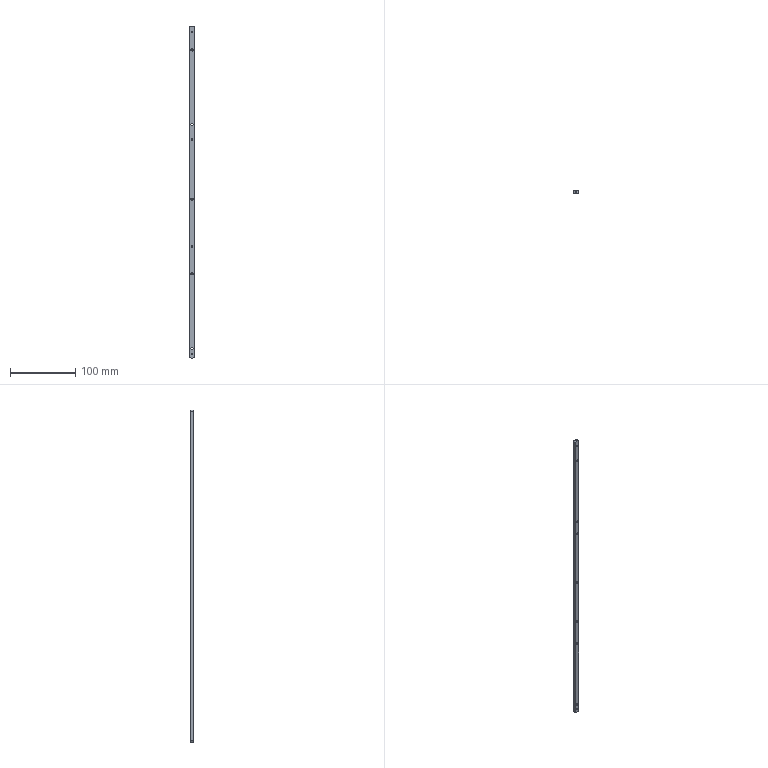Part | NX | 1 solid | 33 faces | box 7 x 5 x 507 mm | volume 17027 mm3 | cylinder 18 | plane 11 | cone 4 | commonest cylinder face diameters 3.4 x5 6 x5 2.5 x4 4 x4
STEP:
#1=CARTESIAN_POINT('',(0.,1.6,220.));
#2=VERTEX_POINT('',#1);
#3=CARTESIAN_POINT('',(0.,1.6,217.));
#4=DIRECTION('',(0.,1.,0.));
#5=DIRECTION('',(0.,0.,1.));
#6=AXIS2_PLACEMENT_3D('',#3,#4,#5);
#7=CIRCLE('',#6,3.);
#8=EDGE_CURVE('',#2,#2,#7,.T.);
#9=ORIENTED_EDGE('',*,*,#8,.T.);
#10=EDGE_LOOP('',(#9));
#11=FACE_BOUND('',#10,.T.);
#12=CARTESIAN_POINT('',(0.,1.6,218.7));
#13=VERTEX_POINT('',#12);
#14=CARTESIAN_POINT('',(0.,1.6,217.));
#15=DIRECTION('',(0.,1.,0.));
#16=DIRECTION('',(0.,0.,1.));
#17=AXIS2_PLACEMENT_3D('',#14,#15,#16);
#18=CIRCLE('',#17,1.7);
#19=EDGE_CURVE('',#13,#13,#18,.T.);
#20=ORIENTED_EDGE('',*,*,#19,.F.);
#21=EDGE_LOOP('',(#20));
#22=FACE_BOUND('',#21,.T.);
#23=CARTESIAN_POINT('',(1.7,1.6,217.));
#24=DIRECTION('',(0.,-1.,0.));
#25=DIRECTION('',(0.,0.,-1.));
#26=AXIS2_PLACEMENT_3D('',#23,#24,#25);
#27=PLANE('',#26);
#28=ADVANCED_FACE('',(#11,#22),#27,.F.);
#29=CARTESIAN_POINT('',(0.,1.6,100.));
#30=VERTEX_POINT('',#29);
#31=CARTESIAN_POINT('',(0.,1.6,103.));
#32=DIRECTION('',(0.,1.,0.));
#33=DIRECTION('',(0.,0.,-1.));
#34=AXIS2_PLACEMENT_3D('',#31,#32,#33);
#35=CIRCLE('',#34,3.);
#36=EDGE_CURVE('',#30,#30,#35,.T.);
#37=ORIENTED_EDGE('',*,*,#36,.T.);
#38=EDGE_LOOP('',(#37));
#39=FACE_BOUND('',#38,.T.);
#40=CARTESIAN_POINT('',(0.,1.6,101.3));
#41=VERTEX_POINT('',#40);
#42=CARTESIAN_POINT('',(0.,1.6,103.));
#43=DIRECTION('',(0.,1.,0.));
#44=DIRECTION('',(0.,0.,-1.));
#45=AXIS2_PLACEMENT_3D('',#42,#43,#44);
#46=CIRCLE('',#45,1.7);
#47=EDGE_CURVE('',#41,#41,#46,.T.);
#48=ORIENTED_EDGE('',*,*,#47,.F.);
#49=EDGE_LOOP('',(#48));
#50=FACE_BOUND('',#49,.T.);
#51=CARTESIAN_POINT('',(1.7,1.6,217.));
#52=DIRECTION('',(0.,-1.,0.));
#53=DIRECTION('',(0.,0.,-1.));
#54=AXIS2_PLACEMENT_3D('',#51,#52,#53);
#55=PLANE('',#54);
#56=ADVANCED_FACE('',(#39,#50),#55,.F.);
#57=CARTESIAN_POINT('',(0.,1.6,-14.));
#58=VERTEX_POINT('',#57);
#59=CARTESIAN_POINT('',(0.,1.6,-11.));
#60=DIRECTION('',(0.,1.,0.));
#61=DIRECTION('',(0.,0.,-1.));
#62=AXIS2_PLACEMENT_3D('',#59,#60,#61);
#63=CIRCLE('',#62,3.);
#64=EDGE_CURVE('',#58,#58,#63,.T.);
#65=ORIENTED_EDGE('',*,*,#64,.T.);
#66=EDGE_LOOP('',(#65));
#67=FACE_BOUND('',#66,.T.);
#68=CARTESIAN_POINT('',(0.,1.6,-12.7));
#69=VERTEX_POINT('',#68);
#70=CARTESIAN_POINT('',(0.,1.6,-11.));
#71=DIRECTION('',(0.,1.,0.));
#72=DIRECTION('',(0.,0.,-1.));
#73=AXIS2_PLACEMENT_3D('',#70,#71,#72);
#74=CIRCLE('',#73,1.7);
#75=EDGE_CURVE('',#69,#69,#74,.T.);
#76=ORIENTED_EDGE('',*,*,#75,.F.);
#77=EDGE_LOOP('',(#76));
#78=FACE_BOUND('',#77,.T.);
#79=CARTESIAN_POINT('',(1.7,1.6,217.));
#80=DIRECTION('',(0.,-1.,0.));
#81=DIRECTION('',(0.,0.,-1.));
#82=AXIS2_PLACEMENT_3D('',#79,#80,#81);
#83=PLANE('',#82);
#84=ADVANCED_FACE('',(#67,#78),#83,.F.);
#85=CARTESIAN_POINT('',(0.,1.6,-128.));
#86=VERTEX_POINT('',#85);
#87=CARTESIAN_POINT('',(0.,1.6,-125.));
#88=DIRECTION('',(0.,1.,0.));
#89=DIRECTION('',(0.,0.,-1.));
#90=AXIS2_PLACEMENT_3D('',#87,#88,#89);
#91=CIRCLE('',#90,3.);
#92=EDGE_CURVE('',#86,#86,#91,.T.);
#93=ORIENTED_EDGE('',*,*,#92,.T.);
#94=EDGE_LOOP('',(#93));
#95=FACE_BOUND('',#94,.T.);
#96=CARTESIAN_POINT('',(0.,1.6,-126.7));
#97=VERTEX_POINT('',#96);
#98=CARTESIAN_POINT('',(0.,1.6,-125.));
#99=DIRECTION('',(0.,1.,0.));
#100=DIRECTION('',(0.,0.,-1.));
#101=AXIS2_PLACEMENT_3D('',#98,#99,#100);
#102=CIRCLE('',#101,1.7);
#103=EDGE_CURVE('',#97,#97,#102,.T.);
#104=ORIENTED_EDGE('',*,*,#103,.F.);
#105=EDGE_LOOP('',(#104));
#106=FACE_BOUND('',#105,.T.);
#107=CARTESIAN_POINT('',(1.7,1.6,217.));
#108=DIRECTION('',(0.,-1.,0.));
#109=DIRECTION('',(0.,0.,-1.));
#110=AXIS2_PLACEMENT_3D('',#107,#108,#109);
#111=PLANE('',#110);
#112=ADVANCED_FACE('',(#95,#106),#111,.F.);
#113=CARTESIAN_POINT('',(0.,1.6,-242.));
#114=VERTEX_POINT('',#113);
#115=CARTESIAN_POINT('',(0.,1.6,-239.));
#116=DIRECTION('',(0.,1.,0.));
#117=DIRECTION('',(0.,0.,-1.));
#118=AXIS2_PLACEMENT_3D('',#115,#116,#117);
#119=CIRCLE('',#118,3.);
#120=EDGE_CURVE('',#114,#114,#119,.T.);
#121=ORIENTED_EDGE('',*,*,#120,.T.);
#122=EDGE_LOOP('',(#121));
#123=FACE_BOUND('',#122,.T.);
#124=CARTESIAN_POINT('',(0.,1.6,-240.7));
#125=VERTEX_POINT('',#124);
#126=CARTESIAN_POINT('',(0.,1.6,-239.));
#127=DIRECTION('',(0.,1.,0.));
#128=DIRECTION('',(0.,0.,-1.));
#129=AXIS2_PLACEMENT_3D('',#126,#127,#128);
#130=CIRCLE('',#129,1.7);
#131=EDGE_CURVE('',#125,#125,#130,.T.);
#132=ORIENTED_EDGE('',*,*,#131,.F.);
#133=EDGE_LOOP('',(#132));
#134=FACE_BOUND('',#133,.T.);
#135=CARTESIAN_POINT('',(1.7,1.6,217.));
#136=DIRECTION('',(0.,-1.,0.));
#137=DIRECTION('',(0.,0.,-1.));
#138=AXIS2_PLACEMENT_3D('',#135,#136,#137);
#139=PLANE('',#138);
#140=ADVANCED_FACE('',(#123,#134),#139,.F.);
#141=CARTESIAN_POINT('',(-3.5,5.,251.5));
#142=VERTEX_POINT('',#141);
#143=CARTESIAN_POINT('',(-1.5,5.,253.5));
#144=VERTEX_POINT('',#143);
#145=CARTESIAN_POINT('',(-1.5,5.,251.5));
#146=DIRECTION('',(0.,1.,0.));
#147=DIRECTION('',(0.,0.,1.));
#148=AXIS2_PLACEMENT_3D('',#145,#146,#147);
#149=CIRCLE('',#148,2.);
#150=EDGE_CURVE('',#142,#144,#149,.T.);
#151=ORIENTED_EDGE('',*,*,#150,.F.);
#152=CARTESIAN_POINT('',(-3.5,0.,251.5));
#153=VERTEX_POINT('',#152);
#154=CARTESIAN_POINT('',(-3.5,5.,251.5));
#155=DIRECTION('',(0.,1.,0.));
#156=VECTOR('',#155,1000.);
#157=LINE('',#154,#156);
#158=EDGE_CURVE('',#153,#142,#157,.T.);
#159=ORIENTED_EDGE('',*,*,#158,.F.);
#160=CARTESIAN_POINT('',(-1.5,0.,253.5));
#161=VERTEX_POINT('',#160);
#162=CARTESIAN_POINT('',(-1.5,0.,251.5));
#163=DIRECTION('',(0.,-1.,0.));
#164=DIRECTION('',(0.,0.,1.));
#165=AXIS2_PLACEMENT_3D('',#162,#163,#164);
#166=CIRCLE('',#165,2.);
#167=EDGE_CURVE('',#161,#153,#166,.T.);
#168=ORIENTED_EDGE('',*,*,#167,.F.);
#169=CARTESIAN_POINT('',(-1.5,5.,253.5));
#170=DIRECTION('',(0.,-1.,0.));
#171=VECTOR('',#170,1000.);
#172=LINE('',#169,#171);
#173=EDGE_CURVE('',#144,#161,#172,.T.);
#174=ORIENTED_EDGE('',*,*,#173,.F.);
#175=EDGE_LOOP('',(#151,#159,#168,#174));
#176=FACE_BOUND('',#175,.T.);
#177=CARTESIAN_POINT('',(-1.5,5.,251.5));
#178=DIRECTION('',(0.,-1.,0.));
#179=DIRECTION('',(0.,0.,-1.));
#180=AXIS2_PLACEMENT_3D('',#177,#178,#179);
#181=CYLINDRICAL_SURFACE('',#180,2.);
#182=ADVANCED_FACE('',(#176),#181,.T.);
#183=CARTESIAN_POINT('',(1.5,5.,253.5));
#184=VERTEX_POINT('',#183);
#185=CARTESIAN_POINT('',(3.5,5.,251.5));
#186=VERTEX_POINT('',#185);
#187=CARTESIAN_POINT('',(1.5,5.,251.5));
#188=DIRECTION('',(0.,1.,0.));
#189=DIRECTION('',(0.,0.,1.));
#190=AXIS2_PLACEMENT_3D('',#187,#188,#189);
#191=CIRCLE('',#190,2.);
#192=EDGE_CURVE('',#184,#186,#191,.T.);
#193=ORIENTED_EDGE('',*,*,#192,.F.);
#194=CARTESIAN_POINT('',(1.5,0.,253.5));
#195=VERTEX_POINT('',#194);
#196=CARTESIAN_POINT('',(1.5,5.,253.5));
#197=DIRECTION('',(0.,1.,0.));
#198=VECTOR('',#197,1000.);
#199=LINE('',#196,#198);
#200=EDGE_CURVE('',#195,#184,#199,.T.);
#201=ORIENTED_EDGE('',*,*,#200,.F.);
#202=CARTESIAN_POINT('',(3.5,0.,251.5));
#203=VERTEX_POINT('',#202);
#204=CARTESIAN_POINT('',(1.5,0.,251.5));
#205=DIRECTION('',(0.,-1.,0.));
#206=DIRECTION('',(0.,0.,1.));
#207=AXIS2_PLACEMENT_3D('',#204,#205,#206);
#208=CIRCLE('',#207,2.);
#209=EDGE_CURVE('',#203,#195,#208,.T.);
#210=ORIENTED_EDGE('',*,*,#209,.F.);
#211=CARTESIAN_POINT('',(3.5,5.,251.5));
#212=DIRECTION('',(0.,-1.,0.));
#213=VECTOR('',#212,1000.);
#214=LINE('',#211,#213);
#215=EDGE_CURVE('',#186,#203,#214,.T.);
#216=ORIENTED_EDGE('',*,*,#215,.F.);
#217=EDGE_LOOP('',(#193,#201,#210,#216));
#218=FACE_BOUND('',#217,.T.);
#219=CARTESIAN_POINT('',(1.5,5.,251.5));
#220=DIRECTION('',(0.,-1.,0.));
#221=DIRECTION('',(0.,0.,-1.));
#222=AXIS2_PLACEMENT_3D('',#219,#220,#221);
#223=CYLINDRICAL_SURFACE('',#222,2.);
#224=ADVANCED_FACE('',(#218),#223,.T.);
#225=CARTESIAN_POINT('',(3.5,5.,-251.5));
#226=VERTEX_POINT('',#225);
#227=CARTESIAN_POINT('',(1.5,5.,-253.5));
#228=VERTEX_POINT('',#227);
#229=CARTESIAN_POINT('',(1.5,5.,-251.5));
#230=DIRECTION('',(0.,1.,0.));
#231=DIRECTION('',(0.,0.,1.));
#232=AXIS2_PLACEMENT_3D('',#229,#230,#231);
#233=CIRCLE('',#232,2.);
#234=EDGE_CURVE('',#226,#228,#233,.T.);
#235=ORIENTED_EDGE('',*,*,#234,.F.);
#236=CARTESIAN_POINT('',(3.5,0.,-251.5));
#237=VERTEX_POINT('',#236);
#238=CARTESIAN_POINT('',(3.5,5.,-251.5));
#239=DIRECTION('',(0.,1.,0.));
#240=VECTOR('',#239,1000.);
#241=LINE('',#238,#240);
#242=EDGE_CURVE('',#237,#226,#241,.T.);
#243=ORIENTED_EDGE('',*,*,#242,.F.);
#244=CARTESIAN_POINT('',(1.5,0.,-253.5));
#245=VERTEX_POINT('',#244);
#246=CARTESIAN_POINT('',(1.5,0.,-251.5));
#247=DIRECTION('',(0.,-1.,0.));
#248=DIRECTION('',(0.,0.,1.));
#249=AXIS2_PLACEMENT_3D('',#246,#247,#248);
#250=CIRCLE('',#249,2.);
#251=EDGE_CURVE('',#245,#237,#250,.T.);
#252=ORIENTED_EDGE('',*,*,#251,.F.);
#253=CARTESIAN_POINT('',(1.5,5.,-253.5));
#254=DIRECTION('',(0.,-1.,0.));
#255=VECTOR('',#254,1000.);
#256=LINE('',#253,#255);
#257=EDGE_CURVE('',#228,#245,#256,.T.);
#258=ORIENTED_EDGE('',*,*,#257,.F.);
#259=EDGE_LOOP('',(#235,#243,#252,#258));
#260=FACE_BOUND('',#259,.T.);
#261=CARTESIAN_POINT('',(1.5,5.,-251.5));
#262=DIRECTION('',(0.,-1.,0.));
#263=DIRECTION('',(0.,0.,-1.));
#264=AXIS2_PLACEMENT_3D('',#261,#262,#263);
#265=CYLINDRICAL_SURFACE('',#264,2.);
#266=ADVANCED_FACE('',(#260),#265,.T.);
#267=CARTESIAN_POINT('',(-1.5,5.,-253.5));
#268=VERTEX_POINT('',#267);
#269=CARTESIAN_POINT('',(-3.5,5.,-251.5));
#270=VERTEX_POINT('',#269);
#271=CARTESIAN_POINT('',(-1.5,5.,-251.5));
#272=DIRECTION('',(0.,1.,0.));
#273=DIRECTION('',(0.,0.,1.));
#274=AXIS2_PLACEMENT_3D('',#271,#272,#273);
#275=CIRCLE('',#274,2.);
#276=EDGE_CURVE('',#268,#270,#275,.T.);
#277=ORIENTED_EDGE('',*,*,#276,.F.);
#278=CARTESIAN_POINT('',(-1.5,0.,-253.5));
#279=VERTEX_POINT('',#278);
#280=CARTESIAN_POINT('',(-1.5,5.,-253.5));
#281=DIRECTION('',(0.,1.,0.));
#282=VECTOR('',#281,1000.);
#283=LINE('',#280,#282);
#284=EDGE_CURVE('',#279,#268,#283,.T.);
#285=ORIENTED_EDGE('',*,*,#284,.F.);
#286=CARTESIAN_POINT('',(-3.5,0.,-251.5));
#287=VERTEX_POINT('',#286);
#288=CARTESIAN_POINT('',(-1.5,0.,-251.5));
#289=DIRECTION('',(0.,-1.,0.));
#290=DIRECTION('',(0.,0.,1.));
#291=AXIS2_PLACEMENT_3D('',#288,#289,#290);
#292=CIRCLE('',#291,2.);
#293=EDGE_CURVE('',#287,#279,#292,.T.);
#294=ORIENTED_EDGE('',*,*,#293,.F.);
#295=CARTESIAN_POINT('',(-3.5,5.,-251.5));
#296=DIRECTION('',(0.,-1.,0.));
#297=VECTOR('',#296,1000.);
#298=LINE('',#295,#297);
#299=EDGE_CURVE('',#270,#287,#298,.T.);
#300=ORIENTED_EDGE('',*,*,#299,.F.);
#301=EDGE_LOOP('',(#277,#285,#294,#300));
#302=FACE_BOUND('',#301,.T.);
#303=CARTESIAN_POINT('',(-1.5,5.,-251.5));
#304=DIRECTION('',(0.,-1.,0.));
#305=DIRECTION('',(0.,0.,-1.));
#306=AXIS2_PLACEMENT_3D('',#303,#304,#305);
#307=CYLINDRICAL_SURFACE('',#306,2.);
#308=ADVANCED_FACE('',(#302),#307,.T.);
#309=CARTESIAN_POINT('',(-3.5,0.,253.5));
#310=DIRECTION('',(0.,0.,1.));
#311=VECTOR('',#310,1000.);
#312=LINE('',#309,#311);
#313=EDGE_CURVE('',#287,#153,#312,.T.);
#314=ORIENTED_EDGE('',*,*,#313,.F.);
#315=ORIENTED_EDGE('',*,*,#293,.T.);
#316=CARTESIAN_POINT('',(3.5,0.,-253.5));
#317=DIRECTION('',(-1.,0.,0.));
#318=VECTOR('',#317,1000.);
#319=LINE('',#316,#318);
#320=EDGE_CURVE('',#245,#279,#319,.T.);
#321=ORIENTED_EDGE('',*,*,#320,.F.);
#322=ORIENTED_EDGE('',*,*,#251,.T.);
#323=CARTESIAN_POINT('',(3.5,0.,253.5));
#324=DIRECTION('',(0.,0.,-1.));
#325=VECTOR('',#324,1000.);
#326=LINE('',#323,#325);
#327=EDGE_CURVE('',#203,#237,#326,.T.);
#328=ORIENTED_EDGE('',*,*,#327,.F.);
#329=ORIENTED_EDGE('',*,*,#209,.T.);
#330=CARTESIAN_POINT('',(3.5,0.,253.5));
#331=DIRECTION('',(1.,0.,0.));
#332=VECTOR('',#331,1000.);
#333=LINE('',#330,#332);
#334=EDGE_CURVE('',#161,#195,#333,.T.);
#335=ORIENTED_EDGE('',*,*,#334,.F.);
#336=ORIENTED_EDGE('',*,*,#167,.T.);
#337=EDGE_LOOP('',(#314,#315,#321,#322,#328,#329,#335,#336));
#338=FACE_BOUND('',#337,.T.);
#339=CARTESIAN_POINT('',(0.,0.,-246.25));
#340=VERTEX_POINT('',#339);
#341=CARTESIAN_POINT('',(0.,0.,-247.5));
#342=DIRECTION('',(0.,1.,0.));
#343=DIRECTION('',(0.,0.,1.));
#344=AXIS2_PLACEMENT_3D('',#341,#342,#343);
#345=CIRCLE('',#344,1.25);
#346=EDGE_CURVE('',#340,#340,#345,.T.);
#347=ORIENTED_EDGE('',*,*,#346,.T.);
#348=EDGE_LOOP('',(#347));
#349=FACE_BOUND('',#348,.T.);
#350=CARTESIAN_POINT('',(0.,0.,245.75));
#351=VERTEX_POINT('',#350);
#352=CARTESIAN_POINT('',(0.,0.,244.5));
#353=DIRECTION('',(0.,1.,0.));
#354=DIRECTION('',(0.,0.,1.));
#355=AXIS2_PLACEMENT_3D('',#352,#353,#354);
#356=CIRCLE('',#355,1.25);
#357=EDGE_CURVE('',#351,#351,#356,.T.);
#358=ORIENTED_EDGE('',*,*,#357,.T.);
#359=EDGE_LOOP('',(#358));
#360=FACE_BOUND('',#359,.T.);
#361=CARTESIAN_POINT('',(0.,0.,-82.25));
#362=VERTEX_POINT('',#361);
#363=CARTESIAN_POINT('',(0.,0.,-83.5));
#364=DIRECTION('',(0.,1.,0.));
#365=DIRECTION('',(0.,0.,1.));
#366=AXIS2_PLACEMENT_3D('',#363,#364,#365);
#367=CIRCLE('',#366,1.25);
#368=EDGE_CURVE('',#362,#362,#367,.T.);
#369=ORIENTED_EDGE('',*,*,#368,.T.);
#370=EDGE_LOOP('',(#369));
#371=FACE_BOUND('',#370,.T.);
#372=CARTESIAN_POINT('',(0.,0.,81.75));
#373=VERTEX_POINT('',#372);
#374=CARTESIAN_POINT('',(0.,0.,80.5));
#375=DIRECTION('',(0.,1.,0.));
#376=DIRECTION('',(0.,0.,1.));
#377=AXIS2_PLACEMENT_3D('',#374,#375,#376);
#378=CIRCLE('',#377,1.25);
#379=EDGE_CURVE('',#373,#373,#378,.T.);
#380=ORIENTED_EDGE('',*,*,#379,.T.);
#381=EDGE_LOOP('',(#380));
#382=FACE_BOUND('',#381,.T.);
#383=CARTESIAN_POINT('',(0.,0.,-237.3));
#384=VERTEX_POINT('',#383);
#385=CARTESIAN_POINT('',(0.,0.,-239.));
#386=DIRECTION('',(0.,1.,0.));
#387=DIRECTION('',(0.,0.,1.));
#388=AXIS2_PLACEMENT_3D('',#385,#386,#387);
#389=CIRCLE('',#388,1.7);
#390=EDGE_CURVE('',#384,#384,#389,.T.);
#391=ORIENTED_EDGE('',*,*,#390,.T.);
#392=EDGE_LOOP('',(#391));
#393=FACE_BOUND('',#392,.T.);
#394=CARTESIAN_POINT('',(0.,0.,-123.3));
#395=VERTEX_POINT('',#394);
#396=CARTESIAN_POINT('',(0.,0.,-125.));
#397=DIRECTION('',(0.,1.,0.));
#398=DIRECTION('',(0.,0.,1.));
#399=AXIS2_PLACEMENT_3D('',#396,#397,#398);
#400=CIRCLE('',#399,1.7);
#401=EDGE_CURVE('',#395,#395,#400,.T.);
#402=ORIENTED_EDGE('',*,*,#401,.T.);
#403=EDGE_LOOP('',(#402));
#404=FACE_BOUND('',#403,.T.);
#405=CARTESIAN_POINT('',(0.,0.,-9.3));
#406=VERTEX_POINT('',#405);
#407=CARTESIAN_POINT('',(0.,0.,-11.));
#408=DIRECTION('',(0.,1.,0.));
#409=DIRECTION('',(0.,0.,1.));
#410=AXIS2_PLACEMENT_3D('',#407,#408,#409);
#411=CIRCLE('',#410,1.7);
#412=EDGE_CURVE('',#406,#406,#411,.T.);
#413=ORIENTED_EDGE('',*,*,#412,.T.);
#414=EDGE_LOOP('',(#413));
#415=FACE_BOUND('',#414,.T.);
#416=CARTESIAN_POINT('',(0.,0.,104.7));
#417=VERTEX_POINT('',#416);
#418=CARTESIAN_POINT('',(0.,0.,103.));
#419=DIRECTION('',(0.,1.,0.));
#420=DIRECTION('',(0.,0.,1.));
#421=AXIS2_PLACEMENT_3D('',#418,#419,#420);
#422=CIRCLE('',#421,1.7);
#423=EDGE_CURVE('',#417,#417,#422,.T.);
#424=ORIENTED_EDGE('',*,*,#423,.T.);
#425=EDGE_LOOP('',(#424));
#426=FACE_BOUND('',#425,.T.);
#427=CARTESIAN_POINT('',(0.,0.,218.7));
#428=VERTEX_POINT('',#427);
#429=CARTESIAN_POINT('',(0.,0.,217.));
#430=DIRECTION('',(0.,1.,0.));
#431=DIRECTION('',(0.,0.,1.));
#432=AXIS2_PLACEMENT_3D('',#429,#430,#431);
#433=CIRCLE('',#432,1.7);
#434=EDGE_CURVE('',#428,#428,#433,.T.);
#435=ORIENTED_EDGE('',*,*,#434,.T.);
#436=EDGE_LOOP('',(#435));
#437=FACE_BOUND('',#436,.T.);
#438=CARTESIAN_POINT('',(0.,0.,0.));
#439=DIRECTION('',(0.,1.,0.));
#440=DIRECTION('',(0.,0.,1.));
#441=AXIS2_PLACEMENT_3D('',#438,#439,#440);
#442=PLANE('',#441);
#443=ADVANCED_FACE('',(#338,#349,#360,#371,#382,#393,#404,#415,#426,#437),#442,.F.);
#444=CARTESIAN_POINT('',(3.5,5.,-253.5));
#445=DIRECTION('',(-1.,0.,0.));
#446=VECTOR('',#445,1000.);
#447=LINE('',#444,#446);
#448=EDGE_CURVE('',#228,#268,#447,.T.);
#449=ORIENTED_EDGE('',*,*,#448,.T.);
#450=ORIENTED_EDGE('',*,*,#276,.T.);
#451=CARTESIAN_POINT('',(-3.5,5.,253.5));
#452=DIRECTION('',(0.,0.,1.));
#453=VECTOR('',#452,1000.);
#454=LINE('',#451,#453);
#455=EDGE_CURVE('',#270,#142,#454,.T.);
#456=ORIENTED_EDGE('',*,*,#455,.T.);
#457=ORIENTED_EDGE('',*,*,#150,.T.);
#458=CARTESIAN_POINT('',(3.5,5.,253.5));
#459=DIRECTION('',(1.,0.,0.));
#460=VECTOR('',#459,1000.);
#461=LINE('',#458,#460);
#462=EDGE_CURVE('',#144,#184,#461,.T.);
#463=ORIENTED_EDGE('',*,*,#462,.T.);
#464=ORIENTED_EDGE('',*,*,#192,.T.);
#465=CARTESIAN_POINT('',(3.5,5.,253.5));
#466=DIRECTION('',(0.,0.,-1.));
#467=VECTOR('',#466,1000.);
#468=LINE('',#465,#467);
#469=EDGE_CURVE('',#186,#226,#468,.T.);
#470=ORIENTED_EDGE('',*,*,#469,.T.);
#471=ORIENTED_EDGE('',*,*,#234,.T.);
#472=EDGE_LOOP('',(#449,#450,#456,#457,#463,#464,#470,#471));
#473=FACE_BOUND('',#472,.T.);
#474=CARTESIAN_POINT('',(0.,5.,-80.75));
#475=VERTEX_POINT('',#474);
#476=CARTESIAN_POINT('',(0.,5.,-83.5));
#477=DIRECTION('',(0.,-1.,0.));
#478=DIRECTION('',(0.,0.,1.));
#479=AXIS2_PLACEMENT_3D('',#476,#477,#478);
#480=CIRCLE('',#479,2.75);
#481=EDGE_CURVE('',#475,#475,#480,.T.);
#482=ORIENTED_EDGE('',*,*,#481,.T.);
#483=EDGE_LOOP('',(#482));
#484=FACE_BOUND('',#483,.T.);
#485=CARTESIAN_POINT('',(0.,5.,83.25));
#486=VERTEX_POINT('',#485);
#487=CARTESIAN_POINT('',(0.,5.,80.5));
#488=DIRECTION('',(0.,-1.,0.));
#489=DIRECTION('',(0.,0.,1.));
#490=AXIS2_PLACEMENT_3D('',#487,#488,#489);
#491=CIRCLE('',#490,2.75);
#492=EDGE_CURVE('',#486,#486,#491,.T.);
#493=ORIENTED_EDGE('',*,*,#492,.T.);
#494=EDGE_LOOP('',(#493));
#495=FACE_BOUND('',#494,.T.);
#496=CARTESIAN_POINT('',(0.,5.,247.25));
#497=VERTEX_POINT('',#496);
#498=CARTESIAN_POINT('',(0.,5.,244.5));
#499=DIRECTION('',(0.,-1.,0.));
#500=DIRECTION('',(0.,0.,1.));
#501=AXIS2_PLACEMENT_3D('',#498,#499,#500);
#502=CIRCLE('',#501,2.75);
#503=EDGE_CURVE('',#497,#497,#502,.T.);
#504=ORIENTED_EDGE('',*,*,#503,.T.);
#505=EDGE_LOOP('',(#504));
#506=FACE_BOUND('',#505,.T.);
#507=CARTESIAN_POINT('',(0.,5.,-244.75));
#508=VERTEX_POINT('',#507);
#509=CARTESIAN_POINT('',(0.,5.,-247.5));
#510=DIRECTION('',(0.,-1.,0.));
#511=DIRECTION('',(0.,0.,1.));
#512=AXIS2_PLACEMENT_3D('',#509,#510,#511);
#513=CIRCLE('',#512,2.75);
#514=EDGE_CURVE('',#508,#508,#513,.T.);
#515=ORIENTED_EDGE('',*,*,#514,.T.);
#516=EDGE_LOOP('',(#515));
#517=FACE_BOUND('',#516,.T.);
#518=CARTESIAN_POINT('',(0.,5.,-236.));
#519=VERTEX_POINT('',#518);
#520=CARTESIAN_POINT('',(0.,5.,-239.));
#521=DIRECTION('',(0.,1.,0.));
#522=DIRECTION('',(0.,0.,1.));
#523=AXIS2_PLACEMENT_3D('',#520,#521,#522);
#524=CIRCLE('',#523,3.);
#525=EDGE_CURVE('',#519,#519,#524,.T.);
#526=ORIENTED_EDGE('',*,*,#525,.F.);
#527=EDGE_LOOP('',(#526));
#528=FACE_BOUND('',#527,.T.);
#529=CARTESIAN_POINT('',(0.,5.,-122.));
#530=VERTEX_POINT('',#529);
#531=CARTESIAN_POINT('',(0.,5.,-125.));
#532=DIRECTION('',(0.,1.,0.));
#533=DIRECTION('',(0.,0.,1.));
#534=AXIS2_PLACEMENT_3D('',#531,#532,#533);
#535=CIRCLE('',#534,3.);
#536=EDGE_CURVE('',#530,#530,#535,.T.);
#537=ORIENTED_EDGE('',*,*,#536,.F.);
#538=EDGE_LOOP('',(#537));
#539=FACE_BOUND('',#538,.T.);
#540=CARTESIAN_POINT('',(0.,5.,-8.));
#541=VERTEX_POINT('',#540);
#542=CARTESIAN_POINT('',(0.,5.,-11.));
#543=DIRECTION('',(0.,1.,0.));
#544=DIRECTION('',(0.,0.,1.));
#545=AXIS2_PLACEMENT_3D('',#542,#543,#544);
#546=CIRCLE('',#545,3.);
#547=EDGE_CURVE('',#541,#541,#546,.T.);
#548=ORIENTED_EDGE('',*,*,#547,.F.);
#549=EDGE_LOOP('',(#548));
#550=FACE_BOUND('',#549,.T.);
#551=CARTESIAN_POINT('',(0.,5.,106.));
#552=VERTEX_POINT('',#551);
#553=CARTESIAN_POINT('',(0.,5.,103.));
#554=DIRECTION('',(0.,1.,0.));
#555=DIRECTION('',(0.,0.,1.));
#556=AXIS2_PLACEMENT_3D('',#553,#554,#555);
#557=CIRCLE('',#556,3.);
#558=EDGE_CURVE('',#552,#552,#557,.T.);
#559=ORIENTED_EDGE('',*,*,#558,.F.);
#560=EDGE_LOOP('',(#559));
#561=FACE_BOUND('',#560,.T.);
#562=CARTESIAN_POINT('',(0.,5.,220.));
#563=VERTEX_POINT('',#562);
#564=CARTESIAN_POINT('',(0.,5.,217.));
#565=DIRECTION('',(0.,1.,0.));
#566=DIRECTION('',(0.,0.,1.));
#567=AXIS2_PLACEMENT_3D('',#564,#565,#566);
#568=CIRCLE('',#567,3.);
#569=EDGE_CURVE('',#563,#563,#568,.T.);
#570=ORIENTED_EDGE('',*,*,#569,.F.);
#571=EDGE_LOOP('',(#570));
#572=FACE_BOUND('',#571,.T.);
#573=CARTESIAN_POINT('',(0.,5.,0.));
#574=DIRECTION('',(0.,1.,0.));
#575=DIRECTION('',(0.,0.,1.));
#576=AXIS2_PLACEMENT_3D('',#573,#574,#575);
#577=PLANE('',#576);
#578=ADVANCED_FACE('',(#473,#484,#495,#506,#517,#528,#539,#550,#561,#572),#577,.T.);
#579=ORIENTED_EDGE('',*,*,#320,.T.);
#580=ORIENTED_EDGE('',*,*,#284,.T.);
#581=ORIENTED_EDGE('',*,*,#448,.F.);
#582=ORIENTED_EDGE('',*,*,#257,.T.);
#583=EDGE_LOOP('',(#579,#580,#581,#582));
#584=FACE_BOUND('',#583,.T.);
#585=CARTESIAN_POINT('',(3.5,5.,-253.5));
#586=DIRECTION('',(0.,0.,1.));
#587=DIRECTION('',(1.,0.,0.));
#588=AXIS2_PLACEMENT_3D('',#585,#586,#587);
#589=PLANE('',#588);
#590=ADVANCED_FACE('',(#584),#589,.F.);
#591=ORIENTED_EDGE('',*,*,#327,.T.);
#592=ORIENTED_EDGE('',*,*,#242,.T.);
#593=ORIENTED_EDGE('',*,*,#469,.F.);
#594=ORIENTED_EDGE('',*,*,#215,.T.);
#595=EDGE_LOOP('',(#591,#592,#593,#594));
#596=FACE_BOUND('',#595,.T.);
#597=CARTESIAN_POINT('',(3.5,5.,253.5));
#598=DIRECTION('',(-1.,0.,0.));
#599=DIRECTION('',(0.,0.,1.));
#600=AXIS2_PLACEMENT_3D('',#597,#598,#599);
#601=PLANE('',#600);
#602=ADVANCED_FACE('',(#596),#601,.F.);
#603=ORIENTED_EDGE('',*,*,#334,.T.);
#604=ORIENTED_EDGE('',*,*,#200,.T.);
#605=ORIENTED_EDGE('',*,*,#462,.F.);
#606=ORIENTED_EDGE('',*,*,#173,.T.);
#607=EDGE_LOOP('',(#603,#604,#605,#606));
#608=FACE_BOUND('',#607,.T.);
#609=CARTESIAN_POINT('',(3.5,5.,253.5));
#610=DIRECTION('',(0.,0.,-1.));
#611=DIRECTION('',(-1.,0.,0.));
#612=AXIS2_PLACEMENT_3D('',#609,#610,#611);
#613=PLANE('',#612);
#614=ADVANCED_FACE('',(#608),#613,.F.);
#615=ORIENTED_EDGE('',*,*,#455,.F.);
#616=ORIENTED_EDGE('',*,*,#299,.T.);
#617=ORIENTED_EDGE('',*,*,#313,.T.);
#618=ORIENTED_EDGE('',*,*,#158,.T.);
#619=EDGE_LOOP('',(#615,#616,#617,#618));
#620=FACE_BOUND('',#619,.T.);
#621=CARTESIAN_POINT('',(-3.5,5.,253.5));
#622=DIRECTION('',(1.,0.,0.));
#623=DIRECTION('',(0.,0.,-1.));
#624=AXIS2_PLACEMENT_3D('',#621,#622,#623);
#625=PLANE('',#624);
#626=ADVANCED_FACE('',(#620),#625,.F.);
#627=ORIENTED_EDGE('',*,*,#346,.F.);
#628=EDGE_LOOP('',(#627));
#629=FACE_BOUND('',#628,.T.);
#630=CARTESIAN_POINT('',(0.,3.5,-246.25));
#631=VERTEX_POINT('',#630);
#632=CARTESIAN_POINT('',(0.,3.5,-247.5));
#633=DIRECTION('',(0.,1.,0.));
#634=DIRECTION('',(0.,0.,1.));
#635=AXIS2_PLACEMENT_3D('',#632,#633,#634);
#636=CIRCLE('',#635,1.25);
#637=EDGE_CURVE('',#631,#631,#636,.T.);
#638=ORIENTED_EDGE('',*,*,#637,.T.);
#639=EDGE_LOOP('',(#638));
#640=FACE_BOUND('',#639,.T.);
#641=CARTESIAN_POINT('',(0.,5.,-247.5));
#642=DIRECTION('',(0.,1.,0.));
#643=DIRECTION('',(0.,0.,1.));
#644=AXIS2_PLACEMENT_3D('',#641,#642,#643);
#645=CYLINDRICAL_SURFACE('',#644,1.25);
#646=ADVANCED_FACE('',(#629,#640),#645,.F.);
#647=ORIENTED_EDGE('',*,*,#357,.F.);
#648=EDGE_LOOP('',(#647));
#649=FACE_BOUND('',#648,.T.);
#650=CARTESIAN_POINT('',(0.,3.5,245.75));
#651=VERTEX_POINT('',#650);
#652=CARTESIAN_POINT('',(0.,3.5,244.5));
#653=DIRECTION('',(0.,1.,0.));
#654=DIRECTION('',(0.,0.,1.));
#655=AXIS2_PLACEMENT_3D('',#652,#653,#654);
#656=CIRCLE('',#655,1.25);
#657=EDGE_CURVE('',#651,#651,#656,.T.);
#658=ORIENTED_EDGE('',*,*,#657,.T.);
#659=EDGE_LOOP('',(#658));
#660=FACE_BOUND('',#659,.T.);
#661=CARTESIAN_POINT('',(0.,5.,244.5));
#662=DIRECTION('',(0.,1.,0.));
#663=DIRECTION('',(0.,0.,1.));
#664=AXIS2_PLACEMENT_3D('',#661,#662,#663);
#665=CYLINDRICAL_SURFACE('',#664,1.25);
#666=ADVANCED_FACE('',(#649,#660),#665,.F.);
#667=ORIENTED_EDGE('',*,*,#368,.F.);
#668=EDGE_LOOP('',(#667));
#669=FACE_BOUND('',#668,.T.);
#670=CARTESIAN_POINT('',(0.,3.5,-82.25));
#671=VERTEX_POINT('',#670);
#672=CARTESIAN_POINT('',(0.,3.5,-83.5));
#673=DIRECTION('',(0.,1.,0.));
#674=DIRECTION('',(0.,0.,1.));
#675=AXIS2_PLACEMENT_3D('',#672,#673,#674);
#676=CIRCLE('',#675,1.25);
#677=EDGE_CURVE('',#671,#671,#676,.T.);
#678=ORIENTED_EDGE('',*,*,#677,.T.);
#679=EDGE_LOOP('',(#678));
#680=FACE_BOUND('',#679,.T.);
#681=CARTESIAN_POINT('',(0.,5.,-83.5));
#682=DIRECTION('',(0.,1.,0.));
#683=DIRECTION('',(0.,0.,1.));
#684=AXIS2_PLACEMENT_3D('',#681,#682,#683);
#685=CYLINDRICAL_SURFACE('',#684,1.25);
#686=ADVANCED_FACE('',(#669,#680),#685,.F.);
#687=ORIENTED_EDGE('',*,*,#379,.F.);
#688=EDGE_LOOP('',(#687));
#689=FACE_BOUND('',#688,.T.);
#690=CARTESIAN_POINT('',(0.,3.5,81.75));
#691=VERTEX_POINT('',#690);
#692=CARTESIAN_POINT('',(0.,3.5,80.5));
#693=DIRECTION('',(0.,1.,0.));
#694=DIRECTION('',(0.,0.,1.));
#695=AXIS2_PLACEMENT_3D('',#692,#693,#694);
#696=CIRCLE('',#695,1.25);
#697=EDGE_CURVE('',#691,#691,#696,.T.);
#698=ORIENTED_EDGE('',*,*,#697,.T.);
#699=EDGE_LOOP('',(#698));
#700=FACE_BOUND('',#699,.T.);
#701=CARTESIAN_POINT('',(0.,5.,80.5));
#702=DIRECTION('',(0.,1.,0.));
#703=DIRECTION('',(0.,0.,1.));
#704=AXIS2_PLACEMENT_3D('',#701,#702,#703);
#705=CYLINDRICAL_SURFACE('',#704,1.25);
#706=ADVANCED_FACE('',(#689,#700),#705,.F.);
#707=ORIENTED_EDGE('',*,*,#637,.F.);
#708=EDGE_LOOP('',(#707));
#709=FACE_BOUND('',#708,.T.);
#710=ORIENTED_EDGE('',*,*,#514,.F.);
#711=EDGE_LOOP('',(#710));
#712=FACE_BOUND('',#711,.T.);
#713=CARTESIAN_POINT('',(0.,3.5,-247.5));
#714=DIRECTION('',(0.,1.,0.));
#715=DIRECTION('',(0.,0.,1.));
#716=AXIS2_PLACEMENT_3D('',#713,#714,#715);
#717=CONICAL_SURFACE('',#716,1.25,0.7854);
#718=ADVANCED_FACE('',(#709,#712),#717,.F.);
#719=ORIENTED_EDGE('',*,*,#657,.F.);
#720=EDGE_LOOP('',(#719));
#721=FACE_BOUND('',#720,.T.);
#722=ORIENTED_EDGE('',*,*,#503,.F.);
#723=EDGE_LOOP('',(#722));
#724=FACE_BOUND('',#723,.T.);
#725=CARTESIAN_POINT('',(0.,3.5,244.5));
#726=DIRECTION('',(0.,1.,0.));
#727=DIRECTION('',(0.,0.,1.));
#728=AXIS2_PLACEMENT_3D('',#725,#726,#727);
#729=CONICAL_SURFACE('',#728,1.25,0.7854);
#730=ADVANCED_FACE('',(#721,#724),#729,.F.);
#731=ORIENTED_EDGE('',*,*,#697,.F.);
#732=EDGE_LOOP('',(#731));
#733=FACE_BOUND('',#732,.T.);
#734=ORIENTED_EDGE('',*,*,#492,.F.);
#735=EDGE_LOOP('',(#734));
#736=FACE_BOUND('',#735,.T.);
#737=CARTESIAN_POINT('',(0.,3.5,80.5));
#738=DIRECTION('',(0.,1.,0.));
#739=DIRECTION('',(0.,0.,1.));
#740=AXIS2_PLACEMENT_3D('',#737,#738,#739);
#741=CONICAL_SURFACE('',#740,1.25,0.7854);
#742=ADVANCED_FACE('',(#733,#736),#741,.F.);
#743=ORIENTED_EDGE('',*,*,#677,.F.);
#744=EDGE_LOOP('',(#743));
#745=FACE_BOUND('',#744,.T.);
#746=ORIENTED_EDGE('',*,*,#481,.F.);
#747=EDGE_LOOP('',(#746));
#748=FACE_BOUND('',#747,.T.);
#749=CARTESIAN_POINT('',(0.,3.5,-83.5));
#750=DIRECTION('',(0.,1.,0.));
#751=DIRECTION('',(0.,0.,1.));
#752=AXIS2_PLACEMENT_3D('',#749,#750,#751);
#753=CONICAL_SURFACE('',#752,1.25,0.7854);
#754=ADVANCED_FACE('',(#745,#748),#753,.F.);
#755=ORIENTED_EDGE('',*,*,#390,.F.);
#756=EDGE_LOOP('',(#755));
#757=FACE_BOUND('',#756,.T.);
#758=ORIENTED_EDGE('',*,*,#131,.T.);
#759=EDGE_LOOP('',(#758));
#760=FACE_BOUND('',#759,.T.);
#761=CARTESIAN_POINT('',(0.,5.,-239.));
#762=DIRECTION('',(0.,1.,0.));
#763=DIRECTION('',(0.,0.,1.));
#764=AXIS2_PLACEMENT_3D('',#761,#762,#763);
#765=CYLINDRICAL_SURFACE('',#764,1.7);
#766=ADVANCED_FACE('',(#757,#760),#765,.F.);
#767=ORIENTED_EDGE('',*,*,#120,.F.);
#768=EDGE_LOOP('',(#767));
#769=FACE_BOUND('',#768,.T.);
#770=ORIENTED_EDGE('',*,*,#525,.T.);
#771=EDGE_LOOP('',(#770));
#772=FACE_BOUND('',#771,.T.);
#773=CARTESIAN_POINT('',(0.,5.,-239.));
#774=DIRECTION('',(0.,1.,0.));
#775=DIRECTION('',(0.,0.,1.));
#776=AXIS2_PLACEMENT_3D('',#773,#774,#775);
#777=CYLINDRICAL_SURFACE('',#776,3.);
#778=ADVANCED_FACE('',(#769,#772),#777,.F.);
#779=ORIENTED_EDGE('',*,*,#401,.F.);
#780=EDGE_LOOP('',(#779));
#781=FACE_BOUND('',#780,.T.);
#782=ORIENTED_EDGE('',*,*,#103,.T.);
#783=EDGE_LOOP('',(#782));
#784=FACE_BOUND('',#783,.T.);
#785=CARTESIAN_POINT('',(0.,5.,-125.));
#786=DIRECTION('',(0.,1.,0.));
#787=DIRECTION('',(0.,0.,1.));
#788=AXIS2_PLACEMENT_3D('',#785,#786,#787);
#789=CYLINDRICAL_SURFACE('',#788,1.7);
#790=ADVANCED_FACE('',(#781,#784),#789,.F.);
#791=ORIENTED_EDGE('',*,*,#92,.F.);
#792=EDGE_LOOP('',(#791));
#793=FACE_BOUND('',#792,.T.);
#794=ORIENTED_EDGE('',*,*,#536,.T.);
#795=EDGE_LOOP('',(#794));
#796=FACE_BOUND('',#795,.T.);
#797=CARTESIAN_POINT('',(0.,5.,-125.));
#798=DIRECTION('',(0.,1.,0.));
#799=DIRECTION('',(0.,0.,1.));
#800=AXIS2_PLACEMENT_3D('',#797,#798,#799);
#801=CYLINDRICAL_SURFACE('',#800,3.);
#802=ADVANCED_FACE('',(#793,#796),#801,.F.);
#803=ORIENTED_EDGE('',*,*,#412,.F.);
#804=EDGE_LOOP('',(#803));
#805=FACE_BOUND('',#804,.T.);
#806=ORIENTED_EDGE('',*,*,#75,.T.);
#807=EDGE_LOOP('',(#806));
#808=FACE_BOUND('',#807,.T.);
#809=CARTESIAN_POINT('',(0.,5.,-11.));
#810=DIRECTION('',(0.,1.,0.));
#811=DIRECTION('',(0.,0.,1.));
#812=AXIS2_PLACEMENT_3D('',#809,#810,#811);
#813=CYLINDRICAL_SURFACE('',#812,1.7);
#814=ADVANCED_FACE('',(#805,#808),#813,.F.);
#815=ORIENTED_EDGE('',*,*,#64,.F.);
#816=EDGE_LOOP('',(#815));
#817=FACE_BOUND('',#816,.T.);
#818=ORIENTED_EDGE('',*,*,#547,.T.);
#819=EDGE_LOOP('',(#818));
#820=FACE_BOUND('',#819,.T.);
#821=CARTESIAN_POINT('',(0.,5.,-11.));
#822=DIRECTION('',(0.,1.,0.));
#823=DIRECTION('',(0.,0.,1.));
#824=AXIS2_PLACEMENT_3D('',#821,#822,#823);
#825=CYLINDRICAL_SURFACE('',#824,3.);
#826=ADVANCED_FACE('',(#817,#820),#825,.F.);
#827=ORIENTED_EDGE('',*,*,#423,.F.);
#828=EDGE_LOOP('',(#827));
#829=FACE_BOUND('',#828,.T.);
#830=ORIENTED_EDGE('',*,*,#47,.T.);
#831=EDGE_LOOP('',(#830));
#832=FACE_BOUND('',#831,.T.);
#833=CARTESIAN_POINT('',(0.,5.,103.));
#834=DIRECTION('',(0.,1.,0.));
#835=DIRECTION('',(0.,0.,1.));
#836=AXIS2_PLACEMENT_3D('',#833,#834,#835);
#837=CYLINDRICAL_SURFACE('',#836,1.7);
#838=ADVANCED_FACE('',(#829,#832),#837,.F.);
#839=ORIENTED_EDGE('',*,*,#36,.F.);
#840=EDGE_LOOP('',(#839));
#841=FACE_BOUND('',#840,.T.);
#842=ORIENTED_EDGE('',*,*,#558,.T.);
#843=EDGE_LOOP('',(#842));
#844=FACE_BOUND('',#843,.T.);
#845=CARTESIAN_POINT('',(0.,5.,103.));
#846=DIRECTION('',(0.,1.,0.));
#847=DIRECTION('',(0.,0.,1.));
#848=AXIS2_PLACEMENT_3D('',#845,#846,#847);
#849=CYLINDRICAL_SURFACE('',#848,3.);
#850=ADVANCED_FACE('',(#841,#844),#849,.F.);
#851=ORIENTED_EDGE('',*,*,#434,.F.);
#852=EDGE_LOOP('',(#851));
#853=FACE_BOUND('',#852,.T.);
#854=ORIENTED_EDGE('',*,*,#19,.T.);
#855=EDGE_LOOP('',(#854));
#856=FACE_BOUND('',#855,.T.);
#857=CARTESIAN_POINT('',(0.,5.,217.));
#858=DIRECTION('',(0.,1.,0.));
#859=DIRECTION('',(0.,0.,1.));
#860=AXIS2_PLACEMENT_3D('',#857,#858,#859);
#861=CYLINDRICAL_SURFACE('',#860,1.7);
#862=ADVANCED_FACE('',(#853,#856),#861,.F.);
#863=ORIENTED_EDGE('',*,*,#8,.F.);
#864=EDGE_LOOP('',(#863));
#865=FACE_BOUND('',#864,.T.);
#866=ORIENTED_EDGE('',*,*,#569,.T.);
#867=EDGE_LOOP('',(#866));
#868=FACE_BOUND('',#867,.T.);
#869=CARTESIAN_POINT('',(0.,5.,217.));
#870=DIRECTION('',(0.,1.,0.));
#871=DIRECTION('',(0.,0.,1.));
#872=AXIS2_PLACEMENT_3D('',#869,#870,#871);
#873=CYLINDRICAL_SURFACE('',#872,3.);
#874=ADVANCED_FACE('',(#865,#868),#873,.F.);
#875=CLOSED_SHELL('',(#28,#56,#84,#112,#140,#182,#224,#266,#308,#443,#578,#590,#602,#614,#626,#646,#666,#686,#706,#718,#730,#742,#754,#766,#778,#790,#802,#814,#826,#838,#850,#862,#874));
#876=MANIFOLD_SOLID_BREP('',#875);
#877=(LENGTH_UNIT()NAMED_UNIT(*)SI_UNIT(.MILLI.,.METRE.));
#878=UNCERTAINTY_MEASURE_WITH_UNIT(LENGTH_MEASURE(0.00001),#877,'','');
#879=(NAMED_UNIT(*)PLANE_ANGLE_UNIT()SI_UNIT($,.RADIAN.));
#880=(NAMED_UNIT(*)SI_UNIT($,.STERADIAN.)SOLID_ANGLE_UNIT());
#881=(GEOMETRIC_REPRESENTATION_CONTEXT(3)GLOBAL_UNCERTAINTY_ASSIGNED_CONTEXT((#878))GLOBAL_UNIT_ASSIGNED_CONTEXT((#877,#879,#880))REPRESENTATION_CONTEXT('',''));
#882=ADVANCED_BREP_SHAPE_REPRESENTATION('',(#876),#881);